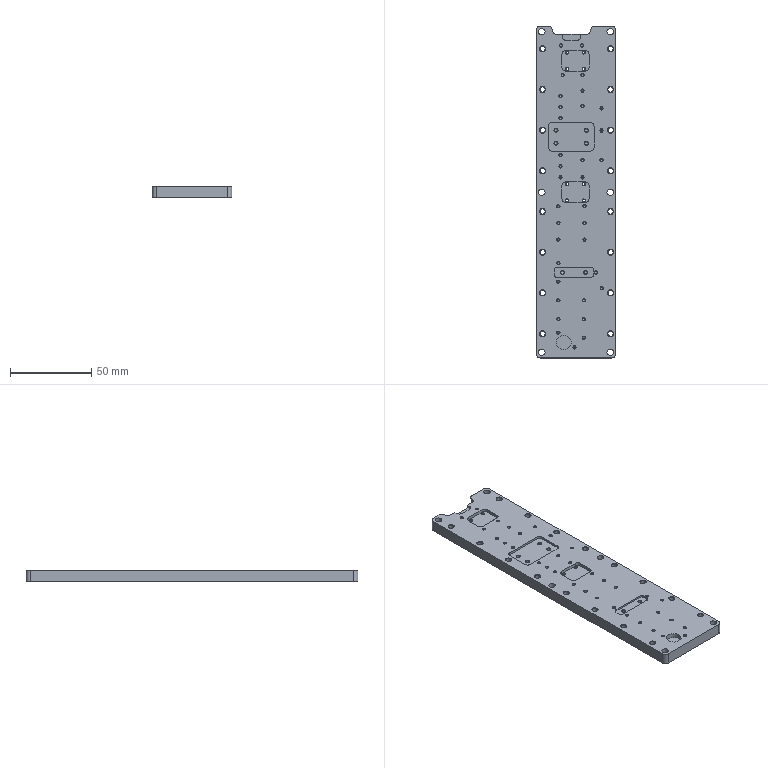Part | STEP file | 53005900 final-stage amplifier red copper | 1 solid | 264 faces | box 49 x 204 x 7 mm | volume 64981 mm3 | cone 132 | cylinder 99 | plane 33 | commonest cylinder face diameters 1.6 x42 5 x22 3.2 x16 4 x10 2.05 x8 9 x1